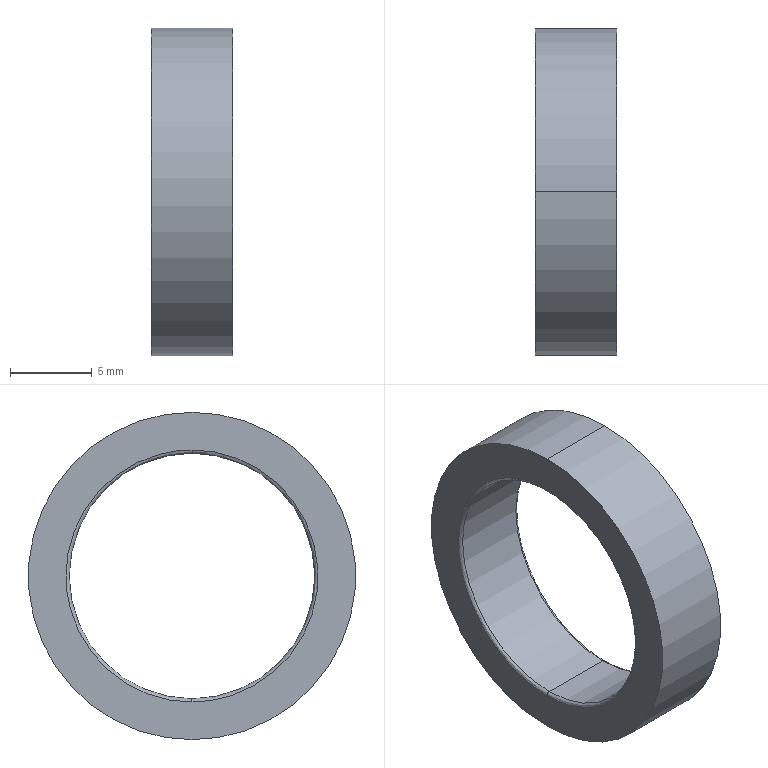Part | STEP file | 0232_Z_UMSB6-20_1 | 1 solid | 10 faces | box 5 x 20 x 20 mm | volume 686.512 mm3 | spline 4 | cylinder 4 | plane 2 | commonest cylinder face diameters 15 x2 20 x2